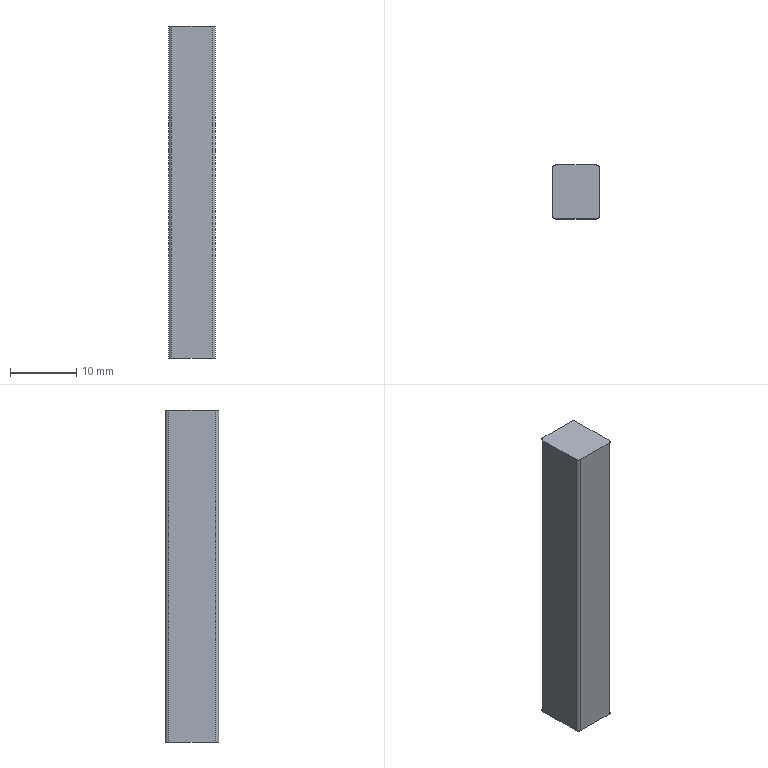Part | NX | features BREP 1 | 1 solid | 10 faces | box 7.03 x 8.05 x 50 mm | volume 2819 mm3 | plane 6 | cylinder 4 | commonest cylinder face diameters 1 x4
STEP:
#1=CARTESIAN_POINT('',(-3.015,4.025,-40.6));
#2=VERTEX_POINT('',#1);
#3=CARTESIAN_POINT('',(-3.515,3.525,-40.6));
#4=VERTEX_POINT('',#3);
#5=CARTESIAN_POINT('',(-3.015,3.525,-40.6));
#6=DIRECTION('',(0.,0.,1.));
#7=DIRECTION('',(1.,0.,0.));
#8=AXIS2_PLACEMENT_3D('',#5,#6,#7);
#9=CIRCLE('',#8,0.5);
#10=EDGE_CURVE('',#2,#4,#9,.T.);
#11=ORIENTED_EDGE('',*,*,#10,.F.);
#12=CARTESIAN_POINT('',(-3.015,4.025,-90.6));
#13=VERTEX_POINT('',#12);
#14=CARTESIAN_POINT('',(-3.015,4.025,-90.6));
#15=DIRECTION('',(0.,0.,1.));
#16=VECTOR('',#15,1000.);
#17=LINE('',#14,#16);
#18=EDGE_CURVE('',#13,#2,#17,.T.);
#19=ORIENTED_EDGE('',*,*,#18,.F.);
#20=CARTESIAN_POINT('',(-3.515,3.525,-90.6));
#21=VERTEX_POINT('',#20);
#22=CARTESIAN_POINT('',(-3.015,3.525,-90.6));
#23=DIRECTION('',(0.,0.,1.));
#24=DIRECTION('',(1.,0.,0.));
#25=AXIS2_PLACEMENT_3D('',#22,#23,#24);
#26=CIRCLE('',#25,0.5);
#27=EDGE_CURVE('',#13,#21,#26,.T.);
#28=ORIENTED_EDGE('',*,*,#27,.T.);
#29=CARTESIAN_POINT('',(-3.515,3.525,-90.6));
#30=DIRECTION('',(0.,0.,1.));
#31=VECTOR('',#30,1000.);
#32=LINE('',#29,#31);
#33=EDGE_CURVE('',#21,#4,#32,.T.);
#34=ORIENTED_EDGE('',*,*,#33,.T.);
#35=EDGE_LOOP('',(#11,#19,#28,#34));
#36=FACE_BOUND('',#35,.T.);
#37=CARTESIAN_POINT('',(-3.015,3.525,-90.6));
#38=DIRECTION('',(0.,0.,1.));
#39=DIRECTION('',(-1.,0.,0.));
#40=AXIS2_PLACEMENT_3D('',#37,#38,#39);
#41=CYLINDRICAL_SURFACE('',#40,0.5);
#42=ADVANCED_FACE('',(#36),#41,.T.);
#43=CARTESIAN_POINT('',(-3.515,-3.525,-40.6));
#44=VERTEX_POINT('',#43);
#45=CARTESIAN_POINT('',(-3.515,-3.525,-40.6));
#46=DIRECTION('',(0.,1.,0.));
#47=VECTOR('',#46,1000.);
#48=LINE('',#45,#47);
#49=EDGE_CURVE('',#44,#4,#48,.T.);
#50=ORIENTED_EDGE('',*,*,#49,.T.);
#51=ORIENTED_EDGE('',*,*,#33,.F.);
#52=CARTESIAN_POINT('',(-3.515,-3.525,-90.6));
#53=VERTEX_POINT('',#52);
#54=CARTESIAN_POINT('',(-3.515,-3.525,-90.6));
#55=DIRECTION('',(0.,1.,0.));
#56=VECTOR('',#55,1000.);
#57=LINE('',#54,#56);
#58=EDGE_CURVE('',#53,#21,#57,.T.);
#59=ORIENTED_EDGE('',*,*,#58,.F.);
#60=CARTESIAN_POINT('',(-3.515,-3.525,-90.6));
#61=DIRECTION('',(0.,0.,1.));
#62=VECTOR('',#61,1000.);
#63=LINE('',#60,#62);
#64=EDGE_CURVE('',#53,#44,#63,.T.);
#65=ORIENTED_EDGE('',*,*,#64,.T.);
#66=EDGE_LOOP('',(#50,#51,#59,#65));
#67=FACE_BOUND('',#66,.T.);
#68=CARTESIAN_POINT('',(-3.515,-3.525,-90.6));
#69=DIRECTION('',(1.,0.,0.));
#70=DIRECTION('',(0.,0.,1.));
#71=AXIS2_PLACEMENT_3D('',#68,#69,#70);
#72=PLANE('',#71);
#73=ADVANCED_FACE('',(#67),#72,.F.);
#74=CARTESIAN_POINT('',(-3.015,-4.025,-40.6));
#75=VERTEX_POINT('',#74);
#76=CARTESIAN_POINT('',(-3.015,-3.525,-40.6));
#77=DIRECTION('',(0.,0.,1.));
#78=DIRECTION('',(1.,0.,0.));
#79=AXIS2_PLACEMENT_3D('',#76,#77,#78);
#80=CIRCLE('',#79,0.5);
#81=EDGE_CURVE('',#44,#75,#80,.T.);
#82=ORIENTED_EDGE('',*,*,#81,.F.);
#83=ORIENTED_EDGE('',*,*,#64,.F.);
#84=CARTESIAN_POINT('',(-3.015,-4.025,-90.6));
#85=VERTEX_POINT('',#84);
#86=CARTESIAN_POINT('',(-3.015,-3.525,-90.6));
#87=DIRECTION('',(0.,0.,1.));
#88=DIRECTION('',(1.,0.,0.));
#89=AXIS2_PLACEMENT_3D('',#86,#87,#88);
#90=CIRCLE('',#89,0.5);
#91=EDGE_CURVE('',#53,#85,#90,.T.);
#92=ORIENTED_EDGE('',*,*,#91,.T.);
#93=CARTESIAN_POINT('',(-3.015,-4.025,-90.6));
#94=DIRECTION('',(0.,0.,1.));
#95=VECTOR('',#94,1000.);
#96=LINE('',#93,#95);
#97=EDGE_CURVE('',#85,#75,#96,.T.);
#98=ORIENTED_EDGE('',*,*,#97,.T.);
#99=EDGE_LOOP('',(#82,#83,#92,#98));
#100=FACE_BOUND('',#99,.T.);
#101=CARTESIAN_POINT('',(-3.015,-3.525,-90.6));
#102=DIRECTION('',(0.,0.,1.));
#103=DIRECTION('',(-1.,0.,0.));
#104=AXIS2_PLACEMENT_3D('',#101,#102,#103);
#105=CYLINDRICAL_SURFACE('',#104,0.5);
#106=ADVANCED_FACE('',(#100),#105,.T.);
#107=CARTESIAN_POINT('',(3.015,-4.025,-40.6));
#108=VERTEX_POINT('',#107);
#109=CARTESIAN_POINT('',(3.015,-4.025,-40.6));
#110=DIRECTION('',(-1.,0.,0.));
#111=VECTOR('',#110,1000.);
#112=LINE('',#109,#111);
#113=EDGE_CURVE('',#108,#75,#112,.T.);
#114=ORIENTED_EDGE('',*,*,#113,.T.);
#115=ORIENTED_EDGE('',*,*,#97,.F.);
#116=CARTESIAN_POINT('',(3.015,-4.025,-90.6));
#117=VERTEX_POINT('',#116);
#118=CARTESIAN_POINT('',(3.015,-4.025,-90.6));
#119=DIRECTION('',(-1.,0.,0.));
#120=VECTOR('',#119,1000.);
#121=LINE('',#118,#120);
#122=EDGE_CURVE('',#117,#85,#121,.T.);
#123=ORIENTED_EDGE('',*,*,#122,.F.);
#124=CARTESIAN_POINT('',(3.015,-4.025,-90.6));
#125=DIRECTION('',(0.,0.,1.));
#126=VECTOR('',#125,1000.);
#127=LINE('',#124,#126);
#128=EDGE_CURVE('',#117,#108,#127,.T.);
#129=ORIENTED_EDGE('',*,*,#128,.T.);
#130=EDGE_LOOP('',(#114,#115,#123,#129));
#131=FACE_BOUND('',#130,.T.);
#132=CARTESIAN_POINT('',(3.015,-4.025,-90.6));
#133=DIRECTION('',(0.,1.,0.));
#134=DIRECTION('',(0.,0.,-1.));
#135=AXIS2_PLACEMENT_3D('',#132,#133,#134);
#136=PLANE('',#135);
#137=ADVANCED_FACE('',(#131),#136,.F.);
#138=CARTESIAN_POINT('',(3.515,-3.525,-40.6));
#139=VERTEX_POINT('',#138);
#140=CARTESIAN_POINT('',(3.015,-3.525,-40.6));
#141=DIRECTION('',(0.,0.,1.));
#142=DIRECTION('',(1.,0.,0.));
#143=AXIS2_PLACEMENT_3D('',#140,#141,#142);
#144=CIRCLE('',#143,0.5);
#145=EDGE_CURVE('',#108,#139,#144,.T.);
#146=ORIENTED_EDGE('',*,*,#145,.F.);
#147=ORIENTED_EDGE('',*,*,#128,.F.);
#148=CARTESIAN_POINT('',(3.515,-3.525,-90.6));
#149=VERTEX_POINT('',#148);
#150=CARTESIAN_POINT('',(3.015,-3.525,-90.6));
#151=DIRECTION('',(0.,0.,1.));
#152=DIRECTION('',(1.,0.,0.));
#153=AXIS2_PLACEMENT_3D('',#150,#151,#152);
#154=CIRCLE('',#153,0.5);
#155=EDGE_CURVE('',#117,#149,#154,.T.);
#156=ORIENTED_EDGE('',*,*,#155,.T.);
#157=CARTESIAN_POINT('',(3.515,-3.525,-90.6));
#158=DIRECTION('',(0.,0.,1.));
#159=VECTOR('',#158,1000.);
#160=LINE('',#157,#159);
#161=EDGE_CURVE('',#149,#139,#160,.T.);
#162=ORIENTED_EDGE('',*,*,#161,.T.);
#163=EDGE_LOOP('',(#146,#147,#156,#162));
#164=FACE_BOUND('',#163,.T.);
#165=CARTESIAN_POINT('',(3.015,-3.525,-90.6));
#166=DIRECTION('',(0.,0.,1.));
#167=DIRECTION('',(-1.,0.,0.));
#168=AXIS2_PLACEMENT_3D('',#165,#166,#167);
#169=CYLINDRICAL_SURFACE('',#168,0.5);
#170=ADVANCED_FACE('',(#164),#169,.T.);
#171=CARTESIAN_POINT('',(3.515,3.525,-40.6));
#172=VERTEX_POINT('',#171);
#173=CARTESIAN_POINT('',(3.515,3.525,-40.6));
#174=DIRECTION('',(0.,-1.,0.));
#175=VECTOR('',#174,1000.);
#176=LINE('',#173,#175);
#177=EDGE_CURVE('',#172,#139,#176,.T.);
#178=ORIENTED_EDGE('',*,*,#177,.T.);
#179=ORIENTED_EDGE('',*,*,#161,.F.);
#180=CARTESIAN_POINT('',(3.515,3.525,-90.6));
#181=VERTEX_POINT('',#180);
#182=CARTESIAN_POINT('',(3.515,3.525,-90.6));
#183=DIRECTION('',(0.,-1.,0.));
#184=VECTOR('',#183,1000.);
#185=LINE('',#182,#184);
#186=EDGE_CURVE('',#181,#149,#185,.T.);
#187=ORIENTED_EDGE('',*,*,#186,.F.);
#188=CARTESIAN_POINT('',(3.515,3.525,-90.6));
#189=DIRECTION('',(0.,0.,1.));
#190=VECTOR('',#189,1000.);
#191=LINE('',#188,#190);
#192=EDGE_CURVE('',#181,#172,#191,.T.);
#193=ORIENTED_EDGE('',*,*,#192,.T.);
#194=EDGE_LOOP('',(#178,#179,#187,#193));
#195=FACE_BOUND('',#194,.T.);
#196=CARTESIAN_POINT('',(3.515,3.525,-90.6));
#197=DIRECTION('',(-1.,0.,0.));
#198=DIRECTION('',(0.,0.,-1.));
#199=AXIS2_PLACEMENT_3D('',#196,#197,#198);
#200=PLANE('',#199);
#201=ADVANCED_FACE('',(#195),#200,.F.);
#202=CARTESIAN_POINT('',(3.015,4.025,-40.6));
#203=VERTEX_POINT('',#202);
#204=CARTESIAN_POINT('',(3.015,3.525,-40.6));
#205=DIRECTION('',(0.,0.,1.));
#206=DIRECTION('',(1.,0.,0.));
#207=AXIS2_PLACEMENT_3D('',#204,#205,#206);
#208=CIRCLE('',#207,0.5);
#209=EDGE_CURVE('',#172,#203,#208,.T.);
#210=ORIENTED_EDGE('',*,*,#209,.F.);
#211=ORIENTED_EDGE('',*,*,#192,.F.);
#212=CARTESIAN_POINT('',(3.015,4.025,-90.6));
#213=VERTEX_POINT('',#212);
#214=CARTESIAN_POINT('',(3.015,3.525,-90.6));
#215=DIRECTION('',(0.,0.,1.));
#216=DIRECTION('',(1.,0.,0.));
#217=AXIS2_PLACEMENT_3D('',#214,#215,#216);
#218=CIRCLE('',#217,0.5);
#219=EDGE_CURVE('',#181,#213,#218,.T.);
#220=ORIENTED_EDGE('',*,*,#219,.T.);
#221=CARTESIAN_POINT('',(3.015,4.025,-90.6));
#222=DIRECTION('',(0.,0.,1.));
#223=VECTOR('',#222,1000.);
#224=LINE('',#221,#223);
#225=EDGE_CURVE('',#213,#203,#224,.T.);
#226=ORIENTED_EDGE('',*,*,#225,.T.);
#227=EDGE_LOOP('',(#210,#211,#220,#226));
#228=FACE_BOUND('',#227,.T.);
#229=CARTESIAN_POINT('',(3.015,3.525,-90.6));
#230=DIRECTION('',(0.,0.,1.));
#231=DIRECTION('',(-1.,0.,0.));
#232=AXIS2_PLACEMENT_3D('',#229,#230,#231);
#233=CYLINDRICAL_SURFACE('',#232,0.5);
#234=ADVANCED_FACE('',(#228),#233,.T.);
#235=CARTESIAN_POINT('',(-3.015,4.025,-40.6));
#236=DIRECTION('',(1.,0.,0.));
#237=VECTOR('',#236,1000.);
#238=LINE('',#235,#237);
#239=EDGE_CURVE('',#2,#203,#238,.T.);
#240=ORIENTED_EDGE('',*,*,#239,.T.);
#241=ORIENTED_EDGE('',*,*,#225,.F.);
#242=CARTESIAN_POINT('',(-3.015,4.025,-90.6));
#243=DIRECTION('',(1.,0.,0.));
#244=VECTOR('',#243,1000.);
#245=LINE('',#242,#244);
#246=EDGE_CURVE('',#13,#213,#245,.T.);
#247=ORIENTED_EDGE('',*,*,#246,.F.);
#248=ORIENTED_EDGE('',*,*,#18,.T.);
#249=EDGE_LOOP('',(#240,#241,#247,#248));
#250=FACE_BOUND('',#249,.T.);
#251=CARTESIAN_POINT('',(-3.015,4.025,-90.6));
#252=DIRECTION('',(0.,-1.,0.));
#253=DIRECTION('',(0.,0.,1.));
#254=AXIS2_PLACEMENT_3D('',#251,#252,#253);
#255=PLANE('',#254);
#256=ADVANCED_FACE('',(#250),#255,.F.);
#257=ORIENTED_EDGE('',*,*,#27,.F.);
#258=ORIENTED_EDGE('',*,*,#246,.T.);
#259=ORIENTED_EDGE('',*,*,#219,.F.);
#260=ORIENTED_EDGE('',*,*,#186,.T.);
#261=ORIENTED_EDGE('',*,*,#155,.F.);
#262=ORIENTED_EDGE('',*,*,#122,.T.);
#263=ORIENTED_EDGE('',*,*,#91,.F.);
#264=ORIENTED_EDGE('',*,*,#58,.T.);
#265=EDGE_LOOP('',(#257,#258,#259,#260,#261,#262,#263,#264));
#266=FACE_BOUND('',#265,.T.);
#267=CARTESIAN_POINT('',(-3.015,3.525,-90.6));
#268=DIRECTION('',(0.,0.,1.));
#269=DIRECTION('',(-1.,0.,0.));
#270=AXIS2_PLACEMENT_3D('',#267,#268,#269);
#271=PLANE('',#270);
#272=ADVANCED_FACE('',(#266),#271,.F.);
#273=ORIENTED_EDGE('',*,*,#10,.T.);
#274=ORIENTED_EDGE('',*,*,#49,.F.);
#275=ORIENTED_EDGE('',*,*,#81,.T.);
#276=ORIENTED_EDGE('',*,*,#113,.F.);
#277=ORIENTED_EDGE('',*,*,#145,.T.);
#278=ORIENTED_EDGE('',*,*,#177,.F.);
#279=ORIENTED_EDGE('',*,*,#209,.T.);
#280=ORIENTED_EDGE('',*,*,#239,.F.);
#281=EDGE_LOOP('',(#273,#274,#275,#276,#277,#278,#279,#280));
#282=FACE_BOUND('',#281,.T.);
#283=CARTESIAN_POINT('',(-3.015,3.525,-40.6));
#284=DIRECTION('',(0.,0.,1.));
#285=DIRECTION('',(-1.,0.,0.));
#286=AXIS2_PLACEMENT_3D('',#283,#284,#285);
#287=PLANE('',#286);
#288=ADVANCED_FACE('',(#282),#287,.T.);
#289=CLOSED_SHELL('',(#42,#73,#106,#137,#170,#201,#234,#256,#272,#288));
#290=MANIFOLD_SOLID_BREP('',#289);
#291=(LENGTH_UNIT()NAMED_UNIT(*)SI_UNIT(.MILLI.,.METRE.));
#292=UNCERTAINTY_MEASURE_WITH_UNIT(LENGTH_MEASURE(0.00001),#291,'','');
#293=(NAMED_UNIT(*)PLANE_ANGLE_UNIT()SI_UNIT($,.RADIAN.));
#294=(NAMED_UNIT(*)SI_UNIT($,.STERADIAN.)SOLID_ANGLE_UNIT());
#295=(GEOMETRIC_REPRESENTATION_CONTEXT(3)GLOBAL_UNCERTAINTY_ASSIGNED_CONTEXT((#292))GLOBAL_UNIT_ASSIGNED_CONTEXT((#291,#293,#294))REPRESENTATION_CONTEXT('',''));
#296=ADVANCED_BREP_SHAPE_REPRESENTATION('',(#290),#295);